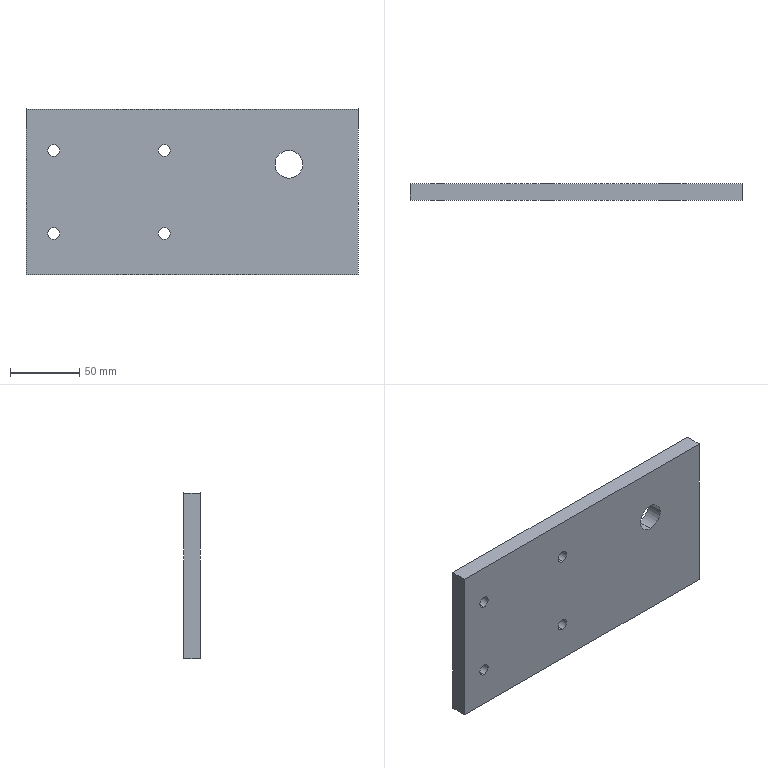Part | SolidWorks | features Extrusion 1 | 1 solid | 16 faces | box 240 x 12 x 120 mm | volume 339106 mm3 | cylinder 10 | plane 6 | commonest cylinder face diameters 8.5 x8 20 x2
STEP:
#1=CARTESIAN_POINT('',(190.,12.,-50.));
#2=VERTEX_POINT('',#1);
#3=CARTESIAN_POINT('',(190.,12.,-30.));
#4=VERTEX_POINT('',#3);
#5=CARTESIAN_POINT('',(190.,12.,-40.));
#6=DIRECTION('',(0.,1.,0.));
#7=DIRECTION('',(0.,0.,1.));
#8=AXIS2_PLACEMENT_3D('',#5,#6,#7);
#9=CIRCLE('',#8,10.);
#10=EDGE_CURVE('',#2,#4,#9,.T.);
#11=ORIENTED_EDGE('',*,*,#10,.T.);
#12=CARTESIAN_POINT('',(190.,0.,-30.));
#13=VERTEX_POINT('',#12);
#14=CARTESIAN_POINT('',(190.,12.,-30.));
#15=DIRECTION('',(0.,-1.,0.));
#16=VECTOR('',#15,1000.);
#17=LINE('',#14,#16);
#18=EDGE_CURVE('',#4,#13,#17,.T.);
#19=ORIENTED_EDGE('',*,*,#18,.T.);
#20=CARTESIAN_POINT('',(190.,0.,-50.));
#21=VERTEX_POINT('',#20);
#22=CARTESIAN_POINT('',(190.,0.,-40.));
#23=DIRECTION('',(0.,1.,0.));
#24=DIRECTION('',(0.,0.,1.));
#25=AXIS2_PLACEMENT_3D('',#22,#23,#24);
#26=CIRCLE('',#25,10.);
#27=EDGE_CURVE('',#21,#13,#26,.T.);
#28=ORIENTED_EDGE('',*,*,#27,.F.);
#29=CARTESIAN_POINT('',(190.,12.,-50.));
#30=DIRECTION('',(0.,-1.,0.));
#31=VECTOR('',#30,1000.);
#32=LINE('',#29,#31);
#33=EDGE_CURVE('',#2,#21,#32,.T.);
#34=ORIENTED_EDGE('',*,*,#33,.F.);
#35=EDGE_LOOP('',(#11,#19,#28,#34));
#36=FACE_OUTER_BOUND('',#35,.T.);
#37=CARTESIAN_POINT('',(190.,12.,-40.));
#38=DIRECTION('',(0.,-1.,0.));
#39=DIRECTION('',(0.,0.,-1.));
#40=AXIS2_PLACEMENT_3D('',#37,#38,#39);
#41=CYLINDRICAL_SURFACE('',#40,10.);
#42=ADVANCED_FACE('',(#36),#41,.F.);
#43=CARTESIAN_POINT('',(100.,12.,-34.25));
#44=VERTEX_POINT('',#43);
#45=CARTESIAN_POINT('',(100.,12.,-25.75));
#46=VERTEX_POINT('',#45);
#47=CARTESIAN_POINT('',(100.,12.,-30.));
#48=DIRECTION('',(0.,1.,0.));
#49=DIRECTION('',(0.,0.,1.));
#50=AXIS2_PLACEMENT_3D('',#47,#48,#49);
#51=CIRCLE('',#50,4.25);
#52=EDGE_CURVE('',#44,#46,#51,.T.);
#53=ORIENTED_EDGE('',*,*,#52,.T.);
#54=CARTESIAN_POINT('',(100.,0.,-25.75));
#55=VERTEX_POINT('',#54);
#56=CARTESIAN_POINT('',(100.,12.,-25.75));
#57=DIRECTION('',(0.,-1.,0.));
#58=VECTOR('',#57,1000.);
#59=LINE('',#56,#58);
#60=EDGE_CURVE('',#46,#55,#59,.T.);
#61=ORIENTED_EDGE('',*,*,#60,.T.);
#62=CARTESIAN_POINT('',(100.,0.,-34.25));
#63=VERTEX_POINT('',#62);
#64=CARTESIAN_POINT('',(100.,0.,-30.));
#65=DIRECTION('',(0.,1.,0.));
#66=DIRECTION('',(0.,0.,1.));
#67=AXIS2_PLACEMENT_3D('',#64,#65,#66);
#68=CIRCLE('',#67,4.25);
#69=EDGE_CURVE('',#63,#55,#68,.T.);
#70=ORIENTED_EDGE('',*,*,#69,.F.);
#71=CARTESIAN_POINT('',(100.,12.,-34.25));
#72=DIRECTION('',(0.,-1.,0.));
#73=VECTOR('',#72,1000.);
#74=LINE('',#71,#73);
#75=EDGE_CURVE('',#44,#63,#74,.T.);
#76=ORIENTED_EDGE('',*,*,#75,.F.);
#77=EDGE_LOOP('',(#53,#61,#70,#76));
#78=FACE_OUTER_BOUND('',#77,.T.);
#79=CARTESIAN_POINT('',(100.,12.,-30.));
#80=DIRECTION('',(0.,-1.,0.));
#81=DIRECTION('',(0.,0.,-1.));
#82=AXIS2_PLACEMENT_3D('',#79,#80,#81);
#83=CYLINDRICAL_SURFACE('',#82,4.25);
#84=ADVANCED_FACE('',(#78),#83,.F.);
#85=CARTESIAN_POINT('',(100.,12.,-94.25));
#86=VERTEX_POINT('',#85);
#87=CARTESIAN_POINT('',(100.,12.,-85.75));
#88=VERTEX_POINT('',#87);
#89=CARTESIAN_POINT('',(100.,12.,-90.));
#90=DIRECTION('',(0.,1.,0.));
#91=DIRECTION('',(0.,0.,1.));
#92=AXIS2_PLACEMENT_3D('',#89,#90,#91);
#93=CIRCLE('',#92,4.25);
#94=EDGE_CURVE('',#86,#88,#93,.T.);
#95=ORIENTED_EDGE('',*,*,#94,.T.);
#96=CARTESIAN_POINT('',(100.,0.,-85.75));
#97=VERTEX_POINT('',#96);
#98=CARTESIAN_POINT('',(100.,12.,-85.75));
#99=DIRECTION('',(0.,-1.,0.));
#100=VECTOR('',#99,1000.);
#101=LINE('',#98,#100);
#102=EDGE_CURVE('',#88,#97,#101,.T.);
#103=ORIENTED_EDGE('',*,*,#102,.T.);
#104=CARTESIAN_POINT('',(100.,0.,-94.25));
#105=VERTEX_POINT('',#104);
#106=CARTESIAN_POINT('',(100.,0.,-90.));
#107=DIRECTION('',(0.,1.,0.));
#108=DIRECTION('',(0.,0.,1.));
#109=AXIS2_PLACEMENT_3D('',#106,#107,#108);
#110=CIRCLE('',#109,4.25);
#111=EDGE_CURVE('',#105,#97,#110,.T.);
#112=ORIENTED_EDGE('',*,*,#111,.F.);
#113=CARTESIAN_POINT('',(100.,12.,-94.25));
#114=DIRECTION('',(0.,-1.,0.));
#115=VECTOR('',#114,1000.);
#116=LINE('',#113,#115);
#117=EDGE_CURVE('',#86,#105,#116,.T.);
#118=ORIENTED_EDGE('',*,*,#117,.F.);
#119=EDGE_LOOP('',(#95,#103,#112,#118));
#120=FACE_OUTER_BOUND('',#119,.T.);
#121=CARTESIAN_POINT('',(100.,12.,-90.));
#122=DIRECTION('',(0.,-1.,0.));
#123=DIRECTION('',(0.,0.,-1.));
#124=AXIS2_PLACEMENT_3D('',#121,#122,#123);
#125=CYLINDRICAL_SURFACE('',#124,4.25);
#126=ADVANCED_FACE('',(#120),#125,.F.);
#127=CARTESIAN_POINT('',(20.,12.,-94.25));
#128=VERTEX_POINT('',#127);
#129=CARTESIAN_POINT('',(20.,12.,-85.75));
#130=VERTEX_POINT('',#129);
#131=CARTESIAN_POINT('',(20.,12.,-90.));
#132=DIRECTION('',(0.,1.,0.));
#133=DIRECTION('',(0.,0.,1.));
#134=AXIS2_PLACEMENT_3D('',#131,#132,#133);
#135=CIRCLE('',#134,4.25);
#136=EDGE_CURVE('',#128,#130,#135,.T.);
#137=ORIENTED_EDGE('',*,*,#136,.T.);
#138=CARTESIAN_POINT('',(20.,0.,-85.75));
#139=VERTEX_POINT('',#138);
#140=CARTESIAN_POINT('',(20.,12.,-85.75));
#141=DIRECTION('',(0.,-1.,0.));
#142=VECTOR('',#141,1000.);
#143=LINE('',#140,#142);
#144=EDGE_CURVE('',#130,#139,#143,.T.);
#145=ORIENTED_EDGE('',*,*,#144,.T.);
#146=CARTESIAN_POINT('',(20.,0.,-94.25));
#147=VERTEX_POINT('',#146);
#148=CARTESIAN_POINT('',(20.,0.,-90.));
#149=DIRECTION('',(0.,1.,0.));
#150=DIRECTION('',(0.,0.,1.));
#151=AXIS2_PLACEMENT_3D('',#148,#149,#150);
#152=CIRCLE('',#151,4.25);
#153=EDGE_CURVE('',#147,#139,#152,.T.);
#154=ORIENTED_EDGE('',*,*,#153,.F.);
#155=CARTESIAN_POINT('',(20.,12.,-94.25));
#156=DIRECTION('',(0.,-1.,0.));
#157=VECTOR('',#156,1000.);
#158=LINE('',#155,#157);
#159=EDGE_CURVE('',#128,#147,#158,.T.);
#160=ORIENTED_EDGE('',*,*,#159,.F.);
#161=EDGE_LOOP('',(#137,#145,#154,#160));
#162=FACE_OUTER_BOUND('',#161,.T.);
#163=CARTESIAN_POINT('',(20.,12.,-90.));
#164=DIRECTION('',(0.,-1.,0.));
#165=DIRECTION('',(0.,0.,-1.));
#166=AXIS2_PLACEMENT_3D('',#163,#164,#165);
#167=CYLINDRICAL_SURFACE('',#166,4.25);
#168=ADVANCED_FACE('',(#162),#167,.F.);
#169=CARTESIAN_POINT('',(20.,12.,-34.25));
#170=VERTEX_POINT('',#169);
#171=CARTESIAN_POINT('',(20.,12.,-25.75));
#172=VERTEX_POINT('',#171);
#173=CARTESIAN_POINT('',(20.,12.,-30.));
#174=DIRECTION('',(0.,1.,0.));
#175=DIRECTION('',(0.,0.,1.));
#176=AXIS2_PLACEMENT_3D('',#173,#174,#175);
#177=CIRCLE('',#176,4.25);
#178=EDGE_CURVE('',#170,#172,#177,.T.);
#179=ORIENTED_EDGE('',*,*,#178,.T.);
#180=CARTESIAN_POINT('',(20.,0.,-25.75));
#181=VERTEX_POINT('',#180);
#182=CARTESIAN_POINT('',(20.,12.,-25.75));
#183=DIRECTION('',(0.,-1.,0.));
#184=VECTOR('',#183,1000.);
#185=LINE('',#182,#184);
#186=EDGE_CURVE('',#172,#181,#185,.T.);
#187=ORIENTED_EDGE('',*,*,#186,.T.);
#188=CARTESIAN_POINT('',(20.,0.,-34.25));
#189=VERTEX_POINT('',#188);
#190=CARTESIAN_POINT('',(20.,0.,-30.));
#191=DIRECTION('',(0.,1.,0.));
#192=DIRECTION('',(0.,0.,1.));
#193=AXIS2_PLACEMENT_3D('',#190,#191,#192);
#194=CIRCLE('',#193,4.25);
#195=EDGE_CURVE('',#189,#181,#194,.T.);
#196=ORIENTED_EDGE('',*,*,#195,.F.);
#197=CARTESIAN_POINT('',(20.,12.,-34.25));
#198=DIRECTION('',(0.,-1.,0.));
#199=VECTOR('',#198,1000.);
#200=LINE('',#197,#199);
#201=EDGE_CURVE('',#170,#189,#200,.T.);
#202=ORIENTED_EDGE('',*,*,#201,.F.);
#203=EDGE_LOOP('',(#179,#187,#196,#202));
#204=FACE_OUTER_BOUND('',#203,.T.);
#205=CARTESIAN_POINT('',(20.,12.,-30.));
#206=DIRECTION('',(0.,-1.,0.));
#207=DIRECTION('',(0.,0.,-1.));
#208=AXIS2_PLACEMENT_3D('',#205,#206,#207);
#209=CYLINDRICAL_SURFACE('',#208,4.25);
#210=ADVANCED_FACE('',(#204),#209,.F.);
#211=CARTESIAN_POINT('',(0.,12.,-120.));
#212=VERTEX_POINT('',#211);
#213=CARTESIAN_POINT('',(0.,12.,0.));
#214=VERTEX_POINT('',#213);
#215=CARTESIAN_POINT('',(0.,12.,0.));
#216=DIRECTION('',(0.,0.,1.));
#217=VECTOR('',#216,1000.);
#218=LINE('',#215,#217);
#219=EDGE_CURVE('',#212,#214,#218,.T.);
#220=ORIENTED_EDGE('',*,*,#219,.T.);
#221=CARTESIAN_POINT('',(240.,12.,0.));
#222=VERTEX_POINT('',#221);
#223=CARTESIAN_POINT('',(0.,12.,0.));
#224=DIRECTION('',(1.,0.,0.));
#225=VECTOR('',#224,1000.);
#226=LINE('',#223,#225);
#227=EDGE_CURVE('',#214,#222,#226,.T.);
#228=ORIENTED_EDGE('',*,*,#227,.T.);
#229=CARTESIAN_POINT('',(240.,12.,-120.));
#230=VERTEX_POINT('',#229);
#231=CARTESIAN_POINT('',(240.,12.,0.));
#232=DIRECTION('',(0.,0.,-1.));
#233=VECTOR('',#232,1000.);
#234=LINE('',#231,#233);
#235=EDGE_CURVE('',#222,#230,#234,.T.);
#236=ORIENTED_EDGE('',*,*,#235,.T.);
#237=CARTESIAN_POINT('',(0.,12.,-120.));
#238=DIRECTION('',(-1.,0.,0.));
#239=VECTOR('',#238,1000.);
#240=LINE('',#237,#239);
#241=EDGE_CURVE('',#230,#212,#240,.T.);
#242=ORIENTED_EDGE('',*,*,#241,.T.);
#243=EDGE_LOOP('',(#220,#228,#236,#242));
#244=FACE_OUTER_BOUND('',#243,.T.);
#245=ORIENTED_EDGE('',*,*,#178,.F.);
#246=CARTESIAN_POINT('',(20.,12.,-30.));
#247=DIRECTION('',(0.,1.,0.));
#248=DIRECTION('',(0.,0.,1.));
#249=AXIS2_PLACEMENT_3D('',#246,#247,#248);
#250=CIRCLE('',#249,4.25);
#251=EDGE_CURVE('',#172,#170,#250,.T.);
#252=ORIENTED_EDGE('',*,*,#251,.F.);
#253=EDGE_LOOP('',(#245,#252));
#254=FACE_BOUND('',#253,.T.);
#255=ORIENTED_EDGE('',*,*,#136,.F.);
#256=CARTESIAN_POINT('',(20.,12.,-90.));
#257=DIRECTION('',(0.,1.,0.));
#258=DIRECTION('',(0.,0.,1.));
#259=AXIS2_PLACEMENT_3D('',#256,#257,#258);
#260=CIRCLE('',#259,4.25);
#261=EDGE_CURVE('',#130,#128,#260,.T.);
#262=ORIENTED_EDGE('',*,*,#261,.F.);
#263=EDGE_LOOP('',(#255,#262));
#264=FACE_BOUND('',#263,.T.);
#265=ORIENTED_EDGE('',*,*,#94,.F.);
#266=CARTESIAN_POINT('',(100.,12.,-90.));
#267=DIRECTION('',(0.,1.,0.));
#268=DIRECTION('',(0.,0.,1.));
#269=AXIS2_PLACEMENT_3D('',#266,#267,#268);
#270=CIRCLE('',#269,4.25);
#271=EDGE_CURVE('',#88,#86,#270,.T.);
#272=ORIENTED_EDGE('',*,*,#271,.F.);
#273=EDGE_LOOP('',(#265,#272));
#274=FACE_BOUND('',#273,.T.);
#275=ORIENTED_EDGE('',*,*,#52,.F.);
#276=CARTESIAN_POINT('',(100.,12.,-30.));
#277=DIRECTION('',(0.,1.,0.));
#278=DIRECTION('',(0.,0.,1.));
#279=AXIS2_PLACEMENT_3D('',#276,#277,#278);
#280=CIRCLE('',#279,4.25);
#281=EDGE_CURVE('',#46,#44,#280,.T.);
#282=ORIENTED_EDGE('',*,*,#281,.F.);
#283=EDGE_LOOP('',(#275,#282));
#284=FACE_BOUND('',#283,.T.);
#285=ORIENTED_EDGE('',*,*,#10,.F.);
#286=CARTESIAN_POINT('',(190.,12.,-40.));
#287=DIRECTION('',(0.,1.,0.));
#288=DIRECTION('',(0.,0.,1.));
#289=AXIS2_PLACEMENT_3D('',#286,#287,#288);
#290=CIRCLE('',#289,10.);
#291=EDGE_CURVE('',#4,#2,#290,.T.);
#292=ORIENTED_EDGE('',*,*,#291,.F.);
#293=EDGE_LOOP('',(#285,#292));
#294=FACE_BOUND('',#293,.T.);
#295=CARTESIAN_POINT('',(0.,12.,0.));
#296=DIRECTION('',(0.,-1.,0.));
#297=DIRECTION('',(0.,0.,-1.));
#298=AXIS2_PLACEMENT_3D('',#295,#296,#297);
#299=PLANE('',#298);
#300=ADVANCED_FACE('',(#244,#254,#264,#274,#284,#294),#299,.F.);
#301=ORIENTED_EDGE('',*,*,#69,.T.);
#302=CARTESIAN_POINT('',(100.,0.,-30.));
#303=DIRECTION('',(0.,1.,0.));
#304=DIRECTION('',(0.,0.,1.));
#305=AXIS2_PLACEMENT_3D('',#302,#303,#304);
#306=CIRCLE('',#305,4.25);
#307=EDGE_CURVE('',#55,#63,#306,.T.);
#308=ORIENTED_EDGE('',*,*,#307,.T.);
#309=EDGE_LOOP('',(#301,#308));
#310=FACE_BOUND('',#309,.T.);
#311=ORIENTED_EDGE('',*,*,#153,.T.);
#312=CARTESIAN_POINT('',(20.,0.,-90.));
#313=DIRECTION('',(0.,1.,0.));
#314=DIRECTION('',(0.,0.,1.));
#315=AXIS2_PLACEMENT_3D('',#312,#313,#314);
#316=CIRCLE('',#315,4.25);
#317=EDGE_CURVE('',#139,#147,#316,.T.);
#318=ORIENTED_EDGE('',*,*,#317,.T.);
#319=EDGE_LOOP('',(#311,#318));
#320=FACE_BOUND('',#319,.T.);
#321=CARTESIAN_POINT('',(0.,0.,-120.));
#322=VERTEX_POINT('',#321);
#323=CARTESIAN_POINT('',(0.,0.,0.));
#324=VERTEX_POINT('',#323);
#325=CARTESIAN_POINT('',(0.,0.,0.));
#326=DIRECTION('',(0.,0.,1.));
#327=VECTOR('',#326,1000.);
#328=LINE('',#325,#327);
#329=EDGE_CURVE('',#322,#324,#328,.T.);
#330=ORIENTED_EDGE('',*,*,#329,.F.);
#331=CARTESIAN_POINT('',(240.,0.,-120.));
#332=VERTEX_POINT('',#331);
#333=CARTESIAN_POINT('',(0.,0.,-120.));
#334=DIRECTION('',(-1.,0.,0.));
#335=VECTOR('',#334,1000.);
#336=LINE('',#333,#335);
#337=EDGE_CURVE('',#332,#322,#336,.T.);
#338=ORIENTED_EDGE('',*,*,#337,.F.);
#339=CARTESIAN_POINT('',(240.,0.,0.));
#340=VERTEX_POINT('',#339);
#341=CARTESIAN_POINT('',(240.,0.,0.));
#342=DIRECTION('',(0.,0.,-1.));
#343=VECTOR('',#342,1000.);
#344=LINE('',#341,#343);
#345=EDGE_CURVE('',#340,#332,#344,.T.);
#346=ORIENTED_EDGE('',*,*,#345,.F.);
#347=CARTESIAN_POINT('',(0.,0.,0.));
#348=DIRECTION('',(1.,0.,0.));
#349=VECTOR('',#348,1000.);
#350=LINE('',#347,#349);
#351=EDGE_CURVE('',#324,#340,#350,.T.);
#352=ORIENTED_EDGE('',*,*,#351,.F.);
#353=EDGE_LOOP('',(#330,#338,#346,#352));
#354=FACE_OUTER_BOUND('',#353,.T.);
#355=ORIENTED_EDGE('',*,*,#195,.T.);
#356=CARTESIAN_POINT('',(20.,0.,-30.));
#357=DIRECTION('',(0.,1.,0.));
#358=DIRECTION('',(0.,0.,1.));
#359=AXIS2_PLACEMENT_3D('',#356,#357,#358);
#360=CIRCLE('',#359,4.25);
#361=EDGE_CURVE('',#181,#189,#360,.T.);
#362=ORIENTED_EDGE('',*,*,#361,.T.);
#363=EDGE_LOOP('',(#355,#362));
#364=FACE_BOUND('',#363,.T.);
#365=ORIENTED_EDGE('',*,*,#111,.T.);
#366=CARTESIAN_POINT('',(100.,0.,-90.));
#367=DIRECTION('',(0.,1.,0.));
#368=DIRECTION('',(0.,0.,1.));
#369=AXIS2_PLACEMENT_3D('',#366,#367,#368);
#370=CIRCLE('',#369,4.25);
#371=EDGE_CURVE('',#97,#105,#370,.T.);
#372=ORIENTED_EDGE('',*,*,#371,.T.);
#373=EDGE_LOOP('',(#365,#372));
#374=FACE_BOUND('',#373,.T.);
#375=ORIENTED_EDGE('',*,*,#27,.T.);
#376=CARTESIAN_POINT('',(190.,0.,-40.));
#377=DIRECTION('',(0.,1.,0.));
#378=DIRECTION('',(0.,0.,1.));
#379=AXIS2_PLACEMENT_3D('',#376,#377,#378);
#380=CIRCLE('',#379,10.);
#381=EDGE_CURVE('',#13,#21,#380,.T.);
#382=ORIENTED_EDGE('',*,*,#381,.T.);
#383=EDGE_LOOP('',(#375,#382));
#384=FACE_BOUND('',#383,.T.);
#385=CARTESIAN_POINT('',(0.,0.,0.));
#386=DIRECTION('',(0.,-1.,0.));
#387=DIRECTION('',(0.,0.,-1.));
#388=AXIS2_PLACEMENT_3D('',#385,#386,#387);
#389=PLANE('',#388);
#390=ADVANCED_FACE('',(#310,#320,#354,#364,#374,#384),#389,.T.);
#391=ORIENTED_EDGE('',*,*,#329,.T.);
#392=CARTESIAN_POINT('',(0.,12.,0.));
#393=DIRECTION('',(0.,-1.,0.));
#394=VECTOR('',#393,1000.);
#395=LINE('',#392,#394);
#396=EDGE_CURVE('',#214,#324,#395,.T.);
#397=ORIENTED_EDGE('',*,*,#396,.F.);
#398=ORIENTED_EDGE('',*,*,#219,.F.);
#399=CARTESIAN_POINT('',(0.,12.,-120.));
#400=DIRECTION('',(0.,-1.,0.));
#401=VECTOR('',#400,1000.);
#402=LINE('',#399,#401);
#403=EDGE_CURVE('',#212,#322,#402,.T.);
#404=ORIENTED_EDGE('',*,*,#403,.T.);
#405=EDGE_LOOP('',(#391,#397,#398,#404));
#406=FACE_OUTER_BOUND('',#405,.T.);
#407=CARTESIAN_POINT('',(0.,12.,0.));
#408=DIRECTION('',(1.,0.,0.));
#409=DIRECTION('',(0.,0.,-1.));
#410=AXIS2_PLACEMENT_3D('',#407,#408,#409);
#411=PLANE('',#410);
#412=ADVANCED_FACE('',(#406),#411,.F.);
#413=ORIENTED_EDGE('',*,*,#351,.T.);
#414=CARTESIAN_POINT('',(240.,12.,0.));
#415=DIRECTION('',(0.,-1.,0.));
#416=VECTOR('',#415,1000.);
#417=LINE('',#414,#416);
#418=EDGE_CURVE('',#222,#340,#417,.T.);
#419=ORIENTED_EDGE('',*,*,#418,.F.);
#420=ORIENTED_EDGE('',*,*,#227,.F.);
#421=ORIENTED_EDGE('',*,*,#396,.T.);
#422=EDGE_LOOP('',(#413,#419,#420,#421));
#423=FACE_OUTER_BOUND('',#422,.T.);
#424=CARTESIAN_POINT('',(0.,12.,0.));
#425=DIRECTION('',(0.,0.,-1.));
#426=DIRECTION('',(-1.,0.,0.));
#427=AXIS2_PLACEMENT_3D('',#424,#425,#426);
#428=PLANE('',#427);
#429=ADVANCED_FACE('',(#423),#428,.F.);
#430=ORIENTED_EDGE('',*,*,#345,.T.);
#431=CARTESIAN_POINT('',(240.,12.,-120.));
#432=DIRECTION('',(0.,-1.,0.));
#433=VECTOR('',#432,1000.);
#434=LINE('',#431,#433);
#435=EDGE_CURVE('',#230,#332,#434,.T.);
#436=ORIENTED_EDGE('',*,*,#435,.F.);
#437=ORIENTED_EDGE('',*,*,#235,.F.);
#438=ORIENTED_EDGE('',*,*,#418,.T.);
#439=EDGE_LOOP('',(#430,#436,#437,#438));
#440=FACE_OUTER_BOUND('',#439,.T.);
#441=CARTESIAN_POINT('',(240.,12.,0.));
#442=DIRECTION('',(-1.,0.,0.));
#443=DIRECTION('',(0.,0.,1.));
#444=AXIS2_PLACEMENT_3D('',#441,#442,#443);
#445=PLANE('',#444);
#446=ADVANCED_FACE('',(#440),#445,.F.);
#447=ORIENTED_EDGE('',*,*,#337,.T.);
#448=ORIENTED_EDGE('',*,*,#403,.F.);
#449=ORIENTED_EDGE('',*,*,#241,.F.);
#450=ORIENTED_EDGE('',*,*,#435,.T.);
#451=EDGE_LOOP('',(#447,#448,#449,#450));
#452=FACE_OUTER_BOUND('',#451,.T.);
#453=CARTESIAN_POINT('',(0.,12.,-120.));
#454=DIRECTION('',(0.,0.,1.));
#455=DIRECTION('',(1.,0.,0.));
#456=AXIS2_PLACEMENT_3D('',#453,#454,#455);
#457=PLANE('',#456);
#458=ADVANCED_FACE('',(#452),#457,.F.);
#459=ORIENTED_EDGE('',*,*,#186,.F.);
#460=ORIENTED_EDGE('',*,*,#251,.T.);
#461=ORIENTED_EDGE('',*,*,#201,.T.);
#462=ORIENTED_EDGE('',*,*,#361,.F.);
#463=EDGE_LOOP('',(#459,#460,#461,#462));
#464=FACE_OUTER_BOUND('',#463,.T.);
#465=CARTESIAN_POINT('',(20.,12.,-30.));
#466=DIRECTION('',(0.,-1.,0.));
#467=DIRECTION('',(0.,0.,-1.));
#468=AXIS2_PLACEMENT_3D('',#465,#466,#467);
#469=CYLINDRICAL_SURFACE('',#468,4.25);
#470=ADVANCED_FACE('',(#464),#469,.F.);
#471=ORIENTED_EDGE('',*,*,#144,.F.);
#472=ORIENTED_EDGE('',*,*,#261,.T.);
#473=ORIENTED_EDGE('',*,*,#159,.T.);
#474=ORIENTED_EDGE('',*,*,#317,.F.);
#475=EDGE_LOOP('',(#471,#472,#473,#474));
#476=FACE_OUTER_BOUND('',#475,.T.);
#477=CARTESIAN_POINT('',(20.,12.,-90.));
#478=DIRECTION('',(0.,-1.,0.));
#479=DIRECTION('',(0.,0.,-1.));
#480=AXIS2_PLACEMENT_3D('',#477,#478,#479);
#481=CYLINDRICAL_SURFACE('',#480,4.25);
#482=ADVANCED_FACE('',(#476),#481,.F.);
#483=ORIENTED_EDGE('',*,*,#102,.F.);
#484=ORIENTED_EDGE('',*,*,#271,.T.);
#485=ORIENTED_EDGE('',*,*,#117,.T.);
#486=ORIENTED_EDGE('',*,*,#371,.F.);
#487=EDGE_LOOP('',(#483,#484,#485,#486));
#488=FACE_OUTER_BOUND('',#487,.T.);
#489=CARTESIAN_POINT('',(100.,12.,-90.));
#490=DIRECTION('',(0.,-1.,0.));
#491=DIRECTION('',(0.,0.,-1.));
#492=AXIS2_PLACEMENT_3D('',#489,#490,#491);
#493=CYLINDRICAL_SURFACE('',#492,4.25);
#494=ADVANCED_FACE('',(#488),#493,.F.);
#495=ORIENTED_EDGE('',*,*,#60,.F.);
#496=ORIENTED_EDGE('',*,*,#281,.T.);
#497=ORIENTED_EDGE('',*,*,#75,.T.);
#498=ORIENTED_EDGE('',*,*,#307,.F.);
#499=EDGE_LOOP('',(#495,#496,#497,#498));
#500=FACE_OUTER_BOUND('',#499,.T.);
#501=CARTESIAN_POINT('',(100.,12.,-30.));
#502=DIRECTION('',(0.,-1.,0.));
#503=DIRECTION('',(0.,0.,-1.));
#504=AXIS2_PLACEMENT_3D('',#501,#502,#503);
#505=CYLINDRICAL_SURFACE('',#504,4.25);
#506=ADVANCED_FACE('',(#500),#505,.F.);
#507=ORIENTED_EDGE('',*,*,#18,.F.);
#508=ORIENTED_EDGE('',*,*,#291,.T.);
#509=ORIENTED_EDGE('',*,*,#33,.T.);
#510=ORIENTED_EDGE('',*,*,#381,.F.);
#511=EDGE_LOOP('',(#507,#508,#509,#510));
#512=FACE_OUTER_BOUND('',#511,.T.);
#513=CARTESIAN_POINT('',(190.,12.,-40.));
#514=DIRECTION('',(0.,-1.,0.));
#515=DIRECTION('',(0.,0.,-1.));
#516=AXIS2_PLACEMENT_3D('',#513,#514,#515);
#517=CYLINDRICAL_SURFACE('',#516,10.);
#518=ADVANCED_FACE('',(#512),#517,.F.);
#519=CLOSED_SHELL('',(#42,#84,#126,#168,#210,#300,#390,#412,#429,#446,#458,#470,#482,#494,#506,#518));
#520=MANIFOLD_SOLID_BREP('',#519);
#521=CARTESIAN_POINT('',(0.,0.,0.));
#522=DIRECTION('',(0.,0.,1.));
#523=DIRECTION('',(1.,0.,0.));
#524=AXIS2_PLACEMENT_3D('',#521,#522,#523);
#525=(LENGTH_UNIT()NAMED_UNIT(*)SI_UNIT(.MILLI.,.METRE.));
#526=UNCERTAINTY_MEASURE_WITH_UNIT(LENGTH_MEASURE(0.00001),#525,'','');
#527=(NAMED_UNIT(*)PLANE_ANGLE_UNIT()SI_UNIT($,.RADIAN.));
#528=(NAMED_UNIT(*)SI_UNIT($,.STERADIAN.)SOLID_ANGLE_UNIT());
#529=(GEOMETRIC_REPRESENTATION_CONTEXT(3)GLOBAL_UNCERTAINTY_ASSIGNED_CONTEXT((#526))GLOBAL_UNIT_ASSIGNED_CONTEXT((#525,#527,#528))REPRESENTATION_CONTEXT('',''));
#530=ADVANCED_BREP_SHAPE_REPRESENTATION('',(#520,#524),#529);